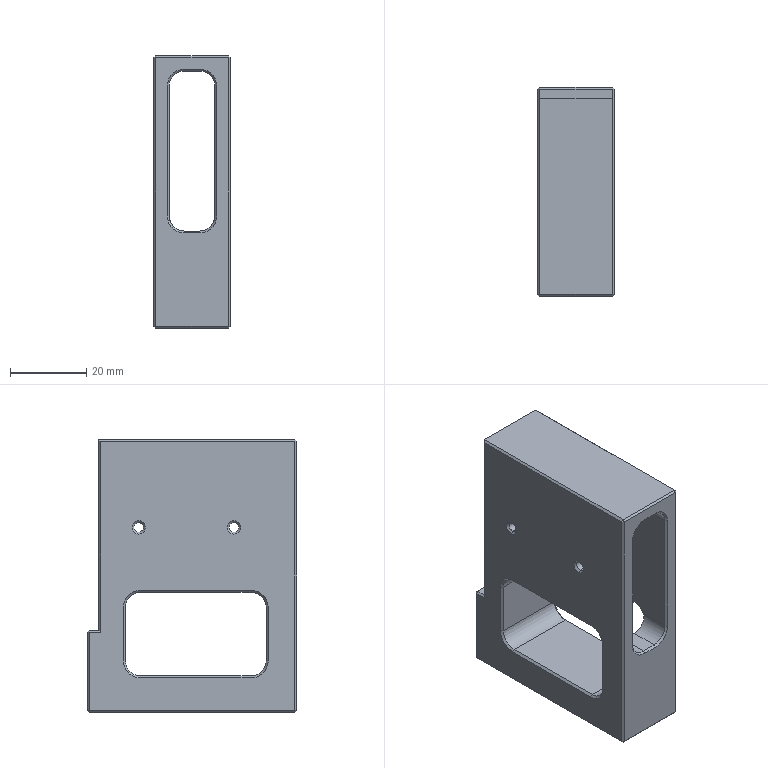Part | STEP file | 10000020502swp000-1 | 1 solid | 109 faces | box 20 x 55 x 71.5 mm | volume 35997 mm3 | plane 54 | cylinder 28 | cone 27 | commonest cylinder face diameters 8 x12 2.5 x8 3 x4 3.3 x4